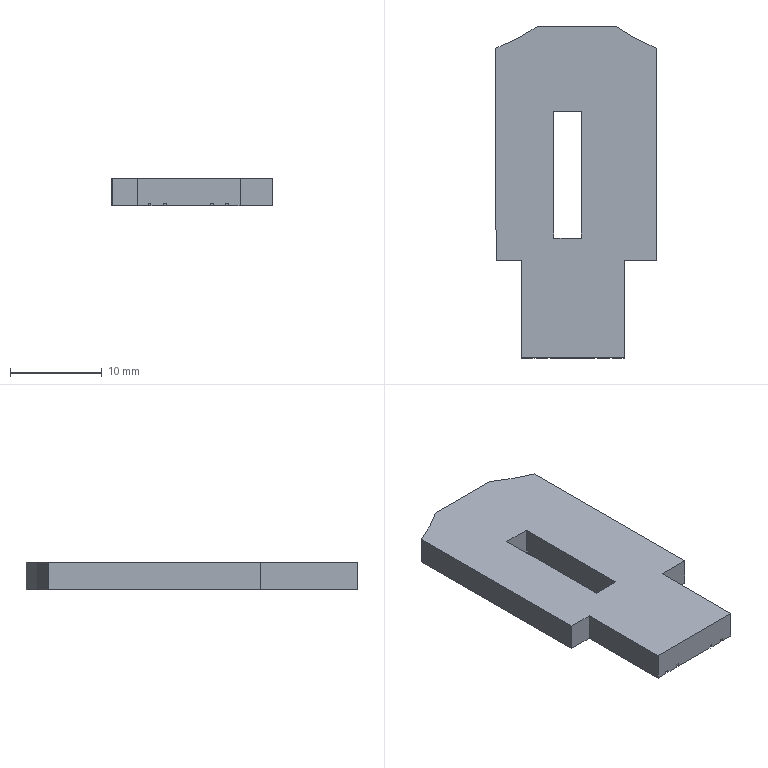Part | SolidWorks | features BaseBody 1 | 1 solid | 62 faces | box 17.454 x 36.156 x 3 mm | volume 1527 mm3 | plane 62